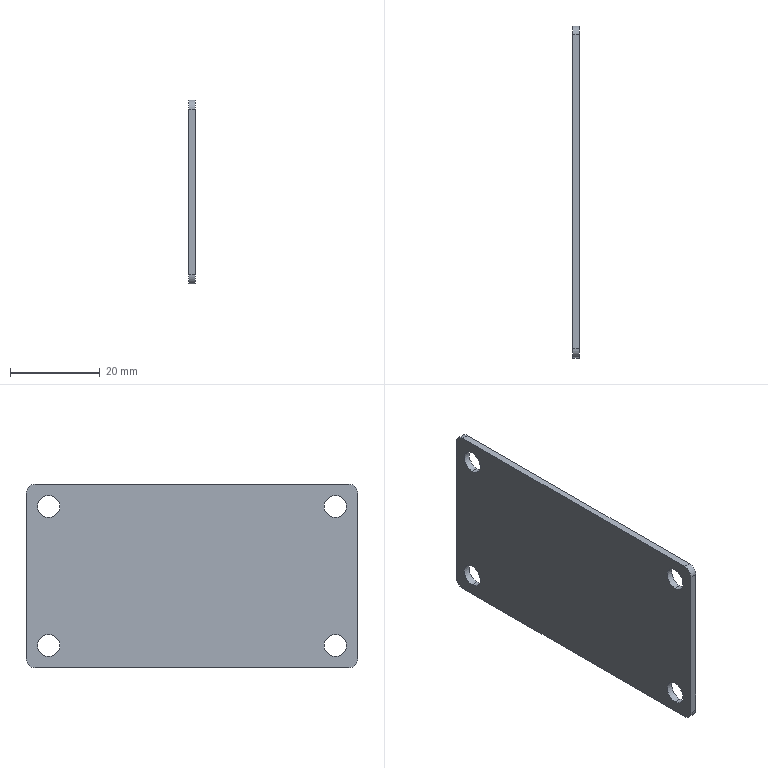Part | NX | features solid 2 | 1 solid | 18 faces | box 1.5 x 74 x 41 mm | volume 4428 mm3 | cylinder 12 | plane 6 | commonest cylinder face diameters 5 x8 4 x4
STEP:
#1=CARTESIAN_POINT('',(-328.,279.,-81.));
#2=VERTEX_POINT('',#1);
#3=CARTESIAN_POINT('',(-328.,277.,-83.));
#4=VERTEX_POINT('',#3);
#5=CARTESIAN_POINT('',(-328.,277.,-81.));
#6=DIRECTION('',(-1.,0.,0.));
#7=DIRECTION('',(0.,0.,-1.));
#8=AXIS2_PLACEMENT_3D('',#5,#6,#7);
#9=CIRCLE('',#8,2.);
#10=EDGE_CURVE('',#2,#4,#9,.T.);
#11=ORIENTED_EDGE('',*,*,#10,.F.);
#12=CARTESIAN_POINT('',(-326.5,279.,-81.));
#13=VERTEX_POINT('',#12);
#14=CARTESIAN_POINT('',(-328.,279.,-81.));
#15=DIRECTION('',(-1.,0.,0.));
#16=VECTOR('',#15,1000.);
#17=LINE('',#14,#16);
#18=EDGE_CURVE('',#13,#2,#17,.T.);
#19=ORIENTED_EDGE('',*,*,#18,.F.);
#20=CARTESIAN_POINT('',(-326.5,277.,-83.));
#21=VERTEX_POINT('',#20);
#22=CARTESIAN_POINT('',(-326.5,277.,-81.));
#23=DIRECTION('',(1.,0.,0.));
#24=DIRECTION('',(0.,0.,-1.));
#25=AXIS2_PLACEMENT_3D('',#22,#23,#24);
#26=CIRCLE('',#25,2.);
#27=EDGE_CURVE('',#21,#13,#26,.T.);
#28=ORIENTED_EDGE('',*,*,#27,.F.);
#29=CARTESIAN_POINT('',(-328.,277.,-83.));
#30=DIRECTION('',(1.,0.,0.));
#31=VECTOR('',#30,1000.);
#32=LINE('',#29,#31);
#33=EDGE_CURVE('',#4,#21,#32,.T.);
#34=ORIENTED_EDGE('',*,*,#33,.F.);
#35=EDGE_LOOP('',(#11,#19,#28,#34));
#36=FACE_BOUND('',#35,.T.);
#37=CARTESIAN_POINT('',(-328.,277.,-81.));
#38=DIRECTION('',(1.,0.,0.));
#39=DIRECTION('',(0.,0.,1.));
#40=AXIS2_PLACEMENT_3D('',#37,#38,#39);
#41=CYLINDRICAL_SURFACE('',#40,2.);
#42=ADVANCED_FACE('',(#36),#41,.T.);
#43=CARTESIAN_POINT('',(-328.,207.,-83.));
#44=VERTEX_POINT('',#43);
#45=CARTESIAN_POINT('',(-328.,205.,-81.));
#46=VERTEX_POINT('',#45);
#47=CARTESIAN_POINT('',(-328.,207.,-81.));
#48=DIRECTION('',(-1.,0.,0.));
#49=DIRECTION('',(0.,0.,-1.));
#50=AXIS2_PLACEMENT_3D('',#47,#48,#49);
#51=CIRCLE('',#50,2.);
#52=EDGE_CURVE('',#44,#46,#51,.T.);
#53=ORIENTED_EDGE('',*,*,#52,.F.);
#54=CARTESIAN_POINT('',(-326.5,207.,-83.));
#55=VERTEX_POINT('',#54);
#56=CARTESIAN_POINT('',(-328.,207.,-83.));
#57=DIRECTION('',(-1.,0.,0.));
#58=VECTOR('',#57,1000.);
#59=LINE('',#56,#58);
#60=EDGE_CURVE('',#55,#44,#59,.T.);
#61=ORIENTED_EDGE('',*,*,#60,.F.);
#62=CARTESIAN_POINT('',(-326.5,205.,-81.));
#63=VERTEX_POINT('',#62);
#64=CARTESIAN_POINT('',(-326.5,207.,-81.));
#65=DIRECTION('',(1.,0.,0.));
#66=DIRECTION('',(0.,0.,-1.));
#67=AXIS2_PLACEMENT_3D('',#64,#65,#66);
#68=CIRCLE('',#67,2.);
#69=EDGE_CURVE('',#63,#55,#68,.T.);
#70=ORIENTED_EDGE('',*,*,#69,.F.);
#71=CARTESIAN_POINT('',(-328.,205.,-81.));
#72=DIRECTION('',(1.,0.,0.));
#73=VECTOR('',#72,1000.);
#74=LINE('',#71,#73);
#75=EDGE_CURVE('',#46,#63,#74,.T.);
#76=ORIENTED_EDGE('',*,*,#75,.F.);
#77=EDGE_LOOP('',(#53,#61,#70,#76));
#78=FACE_BOUND('',#77,.T.);
#79=CARTESIAN_POINT('',(-328.,207.,-81.));
#80=DIRECTION('',(1.,0.,0.));
#81=DIRECTION('',(0.,0.,1.));
#82=AXIS2_PLACEMENT_3D('',#79,#80,#81);
#83=CYLINDRICAL_SURFACE('',#82,2.);
#84=ADVANCED_FACE('',(#78),#83,.T.);
#85=CARTESIAN_POINT('',(-328.,277.,-42.));
#86=VERTEX_POINT('',#85);
#87=CARTESIAN_POINT('',(-328.,279.,-44.));
#88=VERTEX_POINT('',#87);
#89=CARTESIAN_POINT('',(-328.,277.,-44.));
#90=DIRECTION('',(-1.,0.,0.));
#91=DIRECTION('',(0.,0.,-1.));
#92=AXIS2_PLACEMENT_3D('',#89,#90,#91);
#93=CIRCLE('',#92,2.);
#94=EDGE_CURVE('',#86,#88,#93,.T.);
#95=ORIENTED_EDGE('',*,*,#94,.F.);
#96=CARTESIAN_POINT('',(-326.5,277.,-42.));
#97=VERTEX_POINT('',#96);
#98=CARTESIAN_POINT('',(-328.,277.,-42.));
#99=DIRECTION('',(-1.,0.,0.));
#100=VECTOR('',#99,1000.);
#101=LINE('',#98,#100);
#102=EDGE_CURVE('',#97,#86,#101,.T.);
#103=ORIENTED_EDGE('',*,*,#102,.F.);
#104=CARTESIAN_POINT('',(-326.5,279.,-44.));
#105=VERTEX_POINT('',#104);
#106=CARTESIAN_POINT('',(-326.5,277.,-44.));
#107=DIRECTION('',(1.,0.,0.));
#108=DIRECTION('',(0.,0.,-1.));
#109=AXIS2_PLACEMENT_3D('',#106,#107,#108);
#110=CIRCLE('',#109,2.);
#111=EDGE_CURVE('',#105,#97,#110,.T.);
#112=ORIENTED_EDGE('',*,*,#111,.F.);
#113=CARTESIAN_POINT('',(-328.,279.,-44.));
#114=DIRECTION('',(1.,0.,0.));
#115=VECTOR('',#114,1000.);
#116=LINE('',#113,#115);
#117=EDGE_CURVE('',#88,#105,#116,.T.);
#118=ORIENTED_EDGE('',*,*,#117,.F.);
#119=EDGE_LOOP('',(#95,#103,#112,#118));
#120=FACE_BOUND('',#119,.T.);
#121=CARTESIAN_POINT('',(-328.,277.,-44.));
#122=DIRECTION('',(1.,0.,0.));
#123=DIRECTION('',(0.,0.,1.));
#124=AXIS2_PLACEMENT_3D('',#121,#122,#123);
#125=CYLINDRICAL_SURFACE('',#124,2.);
#126=ADVANCED_FACE('',(#120),#125,.T.);
#127=CARTESIAN_POINT('',(-328.,205.,-44.));
#128=VERTEX_POINT('',#127);
#129=CARTESIAN_POINT('',(-328.,207.,-42.));
#130=VERTEX_POINT('',#129);
#131=CARTESIAN_POINT('',(-328.,207.,-44.));
#132=DIRECTION('',(-1.,0.,0.));
#133=DIRECTION('',(0.,0.,-1.));
#134=AXIS2_PLACEMENT_3D('',#131,#132,#133);
#135=CIRCLE('',#134,2.);
#136=EDGE_CURVE('',#128,#130,#135,.T.);
#137=ORIENTED_EDGE('',*,*,#136,.F.);
#138=CARTESIAN_POINT('',(-326.5,205.,-44.));
#139=VERTEX_POINT('',#138);
#140=CARTESIAN_POINT('',(-328.,205.,-44.));
#141=DIRECTION('',(-1.,0.,0.));
#142=VECTOR('',#141,1000.);
#143=LINE('',#140,#142);
#144=EDGE_CURVE('',#139,#128,#143,.T.);
#145=ORIENTED_EDGE('',*,*,#144,.F.);
#146=CARTESIAN_POINT('',(-326.5,207.,-42.));
#147=VERTEX_POINT('',#146);
#148=CARTESIAN_POINT('',(-326.5,207.,-44.));
#149=DIRECTION('',(1.,0.,0.));
#150=DIRECTION('',(0.,0.,-1.));
#151=AXIS2_PLACEMENT_3D('',#148,#149,#150);
#152=CIRCLE('',#151,2.);
#153=EDGE_CURVE('',#147,#139,#152,.T.);
#154=ORIENTED_EDGE('',*,*,#153,.F.);
#155=CARTESIAN_POINT('',(-328.,207.,-42.));
#156=DIRECTION('',(1.,0.,0.));
#157=VECTOR('',#156,1000.);
#158=LINE('',#155,#157);
#159=EDGE_CURVE('',#130,#147,#158,.T.);
#160=ORIENTED_EDGE('',*,*,#159,.F.);
#161=EDGE_LOOP('',(#137,#145,#154,#160));
#162=FACE_BOUND('',#161,.T.);
#163=CARTESIAN_POINT('',(-328.,207.,-44.));
#164=DIRECTION('',(1.,0.,0.));
#165=DIRECTION('',(0.,0.,1.));
#166=AXIS2_PLACEMENT_3D('',#163,#164,#165);
#167=CYLINDRICAL_SURFACE('',#166,2.);
#168=ADVANCED_FACE('',(#162),#167,.T.);
#169=CARTESIAN_POINT('',(-326.5,274.,-49.5));
#170=VERTEX_POINT('',#169);
#171=CARTESIAN_POINT('',(-328.,274.,-49.5));
#172=VERTEX_POINT('',#171);
#173=CARTESIAN_POINT('',(-411.112,274.,-49.5));
#174=DIRECTION('',(1.,0.,0.));
#175=VECTOR('',#174,1000.);
#176=LINE('',#173,#175);
#177=EDGE_CURVE('',#170,#172,#176,.F.);
#178=ORIENTED_EDGE('',*,*,#177,.T.);
#179=CARTESIAN_POINT('',(-328.,274.,-44.5));
#180=VERTEX_POINT('',#179);
#181=CARTESIAN_POINT('',(-328.,274.,-47.));
#182=DIRECTION('',(-1.,0.,0.));
#183=DIRECTION('',(0.,0.,-1.));
#184=AXIS2_PLACEMENT_3D('',#181,#182,#183);
#185=CIRCLE('',#184,2.5);
#186=EDGE_CURVE('',#172,#180,#185,.T.);
#187=ORIENTED_EDGE('',*,*,#186,.T.);
#188=CARTESIAN_POINT('',(-326.5,274.,-44.5));
#189=VERTEX_POINT('',#188);
#190=CARTESIAN_POINT('',(-411.112,274.,-44.5));
#191=DIRECTION('',(1.,0.,0.));
#192=VECTOR('',#191,1000.);
#193=LINE('',#190,#192);
#194=EDGE_CURVE('',#180,#189,#193,.T.);
#195=ORIENTED_EDGE('',*,*,#194,.T.);
#196=CARTESIAN_POINT('',(-326.5,274.,-47.));
#197=DIRECTION('',(1.,0.,0.));
#198=DIRECTION('',(0.,-1.,0.));
#199=AXIS2_PLACEMENT_3D('',#196,#197,#198);
#200=CIRCLE('',#199,2.5);
#201=EDGE_CURVE('',#189,#170,#200,.T.);
#202=ORIENTED_EDGE('',*,*,#201,.T.);
#203=EDGE_LOOP('',(#178,#187,#195,#202));
#204=FACE_BOUND('',#203,.T.);
#205=CARTESIAN_POINT('',(-411.112,274.,-47.));
#206=DIRECTION('',(1.,0.,0.));
#207=DIRECTION('',(0.,0.,1.));
#208=AXIS2_PLACEMENT_3D('',#205,#206,#207);
#209=CYLINDRICAL_SURFACE('',#208,2.5);
#210=ADVANCED_FACE('',(#204),#209,.F.);
#211=CARTESIAN_POINT('',(-326.5,210.,-49.5));
#212=VERTEX_POINT('',#211);
#213=CARTESIAN_POINT('',(-328.,210.,-49.5));
#214=VERTEX_POINT('',#213);
#215=CARTESIAN_POINT('',(-411.112,210.,-49.5));
#216=DIRECTION('',(1.,0.,0.));
#217=VECTOR('',#216,1000.);
#218=LINE('',#215,#217);
#219=EDGE_CURVE('',#212,#214,#218,.F.);
#220=ORIENTED_EDGE('',*,*,#219,.T.);
#221=CARTESIAN_POINT('',(-328.,210.,-44.5));
#222=VERTEX_POINT('',#221);
#223=CARTESIAN_POINT('',(-328.,210.,-47.));
#224=DIRECTION('',(-1.,0.,0.));
#225=DIRECTION('',(0.,0.,-1.));
#226=AXIS2_PLACEMENT_3D('',#223,#224,#225);
#227=CIRCLE('',#226,2.5);
#228=EDGE_CURVE('',#214,#222,#227,.T.);
#229=ORIENTED_EDGE('',*,*,#228,.T.);
#230=CARTESIAN_POINT('',(-326.5,210.,-44.5));
#231=VERTEX_POINT('',#230);
#232=CARTESIAN_POINT('',(-411.112,210.,-44.5));
#233=DIRECTION('',(1.,0.,0.));
#234=VECTOR('',#233,1000.);
#235=LINE('',#232,#234);
#236=EDGE_CURVE('',#222,#231,#235,.T.);
#237=ORIENTED_EDGE('',*,*,#236,.T.);
#238=CARTESIAN_POINT('',(-326.5,210.,-47.));
#239=DIRECTION('',(1.,0.,0.));
#240=DIRECTION('',(0.,-1.,0.));
#241=AXIS2_PLACEMENT_3D('',#238,#239,#240);
#242=CIRCLE('',#241,2.5);
#243=EDGE_CURVE('',#231,#212,#242,.T.);
#244=ORIENTED_EDGE('',*,*,#243,.T.);
#245=EDGE_LOOP('',(#220,#229,#237,#244));
#246=FACE_BOUND('',#245,.T.);
#247=CARTESIAN_POINT('',(-411.112,210.,-47.));
#248=DIRECTION('',(1.,0.,0.));
#249=DIRECTION('',(0.,0.,1.));
#250=AXIS2_PLACEMENT_3D('',#247,#248,#249);
#251=CYLINDRICAL_SURFACE('',#250,2.5);
#252=ADVANCED_FACE('',(#246),#251,.F.);
#253=CARTESIAN_POINT('',(-328.,210.,-80.5));
#254=VERTEX_POINT('',#253);
#255=CARTESIAN_POINT('',(-326.5,210.,-80.5));
#256=VERTEX_POINT('',#255);
#257=CARTESIAN_POINT('',(-411.112,210.,-80.5));
#258=DIRECTION('',(1.,0.,0.));
#259=VECTOR('',#258,1000.);
#260=LINE('',#257,#259);
#261=EDGE_CURVE('',#254,#256,#260,.T.);
#262=ORIENTED_EDGE('',*,*,#261,.F.);
#263=CARTESIAN_POINT('',(-328.,210.,-75.5));
#264=VERTEX_POINT('',#263);
#265=CARTESIAN_POINT('',(-328.,210.,-78.));
#266=DIRECTION('',(-1.,0.,0.));
#267=DIRECTION('',(0.,0.,-1.));
#268=AXIS2_PLACEMENT_3D('',#265,#266,#267);
#269=CIRCLE('',#268,2.5);
#270=EDGE_CURVE('',#254,#264,#269,.T.);
#271=ORIENTED_EDGE('',*,*,#270,.T.);
#272=CARTESIAN_POINT('',(-326.5,210.,-75.5));
#273=VERTEX_POINT('',#272);
#274=CARTESIAN_POINT('',(-411.112,210.,-75.5));
#275=DIRECTION('',(1.,0.,0.));
#276=VECTOR('',#275,1000.);
#277=LINE('',#274,#276);
#278=EDGE_CURVE('',#273,#264,#277,.F.);
#279=ORIENTED_EDGE('',*,*,#278,.F.);
#280=CARTESIAN_POINT('',(-326.5,210.,-78.));
#281=DIRECTION('',(1.,0.,0.));
#282=DIRECTION('',(0.,-1.,0.));
#283=AXIS2_PLACEMENT_3D('',#280,#281,#282);
#284=CIRCLE('',#283,2.5);
#285=EDGE_CURVE('',#273,#256,#284,.T.);
#286=ORIENTED_EDGE('',*,*,#285,.T.);
#287=EDGE_LOOP('',(#262,#271,#279,#286));
#288=FACE_BOUND('',#287,.T.);
#289=CARTESIAN_POINT('',(-411.112,210.,-78.));
#290=DIRECTION('',(1.,0.,0.));
#291=DIRECTION('',(0.,0.,1.));
#292=AXIS2_PLACEMENT_3D('',#289,#290,#291);
#293=CYLINDRICAL_SURFACE('',#292,2.5);
#294=ADVANCED_FACE('',(#288),#293,.F.);
#295=CARTESIAN_POINT('',(-326.5,274.,-80.5));
#296=VERTEX_POINT('',#295);
#297=CARTESIAN_POINT('',(-328.,274.,-80.5));
#298=VERTEX_POINT('',#297);
#299=CARTESIAN_POINT('',(-411.112,274.,-80.5));
#300=DIRECTION('',(1.,0.,0.));
#301=VECTOR('',#300,1000.);
#302=LINE('',#299,#301);
#303=EDGE_CURVE('',#296,#298,#302,.F.);
#304=ORIENTED_EDGE('',*,*,#303,.T.);
#305=CARTESIAN_POINT('',(-328.,274.,-75.5));
#306=VERTEX_POINT('',#305);
#307=CARTESIAN_POINT('',(-328.,274.,-78.));
#308=DIRECTION('',(-1.,0.,0.));
#309=DIRECTION('',(0.,0.,-1.));
#310=AXIS2_PLACEMENT_3D('',#307,#308,#309);
#311=CIRCLE('',#310,2.5);
#312=EDGE_CURVE('',#298,#306,#311,.T.);
#313=ORIENTED_EDGE('',*,*,#312,.T.);
#314=CARTESIAN_POINT('',(-326.5,274.,-75.5));
#315=VERTEX_POINT('',#314);
#316=CARTESIAN_POINT('',(-411.112,274.,-75.5));
#317=DIRECTION('',(1.,0.,0.));
#318=VECTOR('',#317,1000.);
#319=LINE('',#316,#318);
#320=EDGE_CURVE('',#306,#315,#319,.T.);
#321=ORIENTED_EDGE('',*,*,#320,.T.);
#322=CARTESIAN_POINT('',(-326.5,274.,-78.));
#323=DIRECTION('',(1.,0.,0.));
#324=DIRECTION('',(0.,-1.,0.));
#325=AXIS2_PLACEMENT_3D('',#322,#323,#324);
#326=CIRCLE('',#325,2.5);
#327=EDGE_CURVE('',#315,#296,#326,.T.);
#328=ORIENTED_EDGE('',*,*,#327,.T.);
#329=EDGE_LOOP('',(#304,#313,#321,#328));
#330=FACE_BOUND('',#329,.T.);
#331=CARTESIAN_POINT('',(-411.112,274.,-78.));
#332=DIRECTION('',(1.,0.,0.));
#333=DIRECTION('',(0.,0.,1.));
#334=AXIS2_PLACEMENT_3D('',#331,#332,#333);
#335=CYLINDRICAL_SURFACE('',#334,2.5);
#336=ADVANCED_FACE('',(#330),#335,.F.);
#337=ORIENTED_EDGE('',*,*,#327,.F.);
#338=CARTESIAN_POINT('',(-326.5,274.,-78.));
#339=DIRECTION('',(1.,0.,0.));
#340=DIRECTION('',(0.,-1.,0.));
#341=AXIS2_PLACEMENT_3D('',#338,#339,#340);
#342=CIRCLE('',#341,2.5);
#343=EDGE_CURVE('',#296,#315,#342,.T.);
#344=ORIENTED_EDGE('',*,*,#343,.F.);
#345=EDGE_LOOP('',(#337,#344));
#346=FACE_BOUND('',#345,.T.);
#347=ORIENTED_EDGE('',*,*,#285,.F.);
#348=CARTESIAN_POINT('',(-326.5,210.,-78.));
#349=DIRECTION('',(1.,0.,0.));
#350=DIRECTION('',(0.,-1.,0.));
#351=AXIS2_PLACEMENT_3D('',#348,#349,#350);
#352=CIRCLE('',#351,2.5);
#353=EDGE_CURVE('',#256,#273,#352,.T.);
#354=ORIENTED_EDGE('',*,*,#353,.F.);
#355=EDGE_LOOP('',(#347,#354));
#356=FACE_BOUND('',#355,.T.);
#357=ORIENTED_EDGE('',*,*,#243,.F.);
#358=CARTESIAN_POINT('',(-326.5,210.,-47.));
#359=DIRECTION('',(1.,0.,0.));
#360=DIRECTION('',(0.,-1.,0.));
#361=AXIS2_PLACEMENT_3D('',#358,#359,#360);
#362=CIRCLE('',#361,2.5);
#363=EDGE_CURVE('',#212,#231,#362,.T.);
#364=ORIENTED_EDGE('',*,*,#363,.F.);
#365=EDGE_LOOP('',(#357,#364));
#366=FACE_BOUND('',#365,.T.);
#367=ORIENTED_EDGE('',*,*,#201,.F.);
#368=CARTESIAN_POINT('',(-326.5,274.,-47.));
#369=DIRECTION('',(1.,0.,0.));
#370=DIRECTION('',(0.,-1.,0.));
#371=AXIS2_PLACEMENT_3D('',#368,#369,#370);
#372=CIRCLE('',#371,2.5);
#373=EDGE_CURVE('',#170,#189,#372,.T.);
#374=ORIENTED_EDGE('',*,*,#373,.F.);
#375=EDGE_LOOP('',(#367,#374));
#376=FACE_BOUND('',#375,.T.);
#377=CARTESIAN_POINT('',(-326.5,205.,-42.));
#378=DIRECTION('',(0.,1.,0.));
#379=VECTOR('',#378,1000.);
#380=LINE('',#377,#379);
#381=EDGE_CURVE('',#147,#97,#380,.T.);
#382=ORIENTED_EDGE('',*,*,#381,.F.);
#383=ORIENTED_EDGE('',*,*,#153,.T.);
#384=CARTESIAN_POINT('',(-326.5,205.,-83.));
#385=DIRECTION('',(0.,0.,1.));
#386=VECTOR('',#385,1000.);
#387=LINE('',#384,#386);
#388=EDGE_CURVE('',#63,#139,#387,.T.);
#389=ORIENTED_EDGE('',*,*,#388,.F.);
#390=ORIENTED_EDGE('',*,*,#69,.T.);
#391=CARTESIAN_POINT('',(-326.5,279.,-83.));
#392=DIRECTION('',(0.,-1.,0.));
#393=VECTOR('',#392,1000.);
#394=LINE('',#391,#393);
#395=EDGE_CURVE('',#21,#55,#394,.T.);
#396=ORIENTED_EDGE('',*,*,#395,.F.);
#397=ORIENTED_EDGE('',*,*,#27,.T.);
#398=CARTESIAN_POINT('',(-326.5,279.,-42.));
#399=DIRECTION('',(0.,0.,-1.));
#400=VECTOR('',#399,1000.);
#401=LINE('',#398,#400);
#402=EDGE_CURVE('',#105,#13,#401,.T.);
#403=ORIENTED_EDGE('',*,*,#402,.F.);
#404=ORIENTED_EDGE('',*,*,#111,.T.);
#405=EDGE_LOOP('',(#382,#383,#389,#390,#396,#397,#403,#404));
#406=FACE_BOUND('',#405,.T.);
#407=CARTESIAN_POINT('',(-326.5,242.,-62.5));
#408=DIRECTION('',(-1.,0.,0.));
#409=DIRECTION('',(0.,0.,1.));
#410=AXIS2_PLACEMENT_3D('',#407,#408,#409);
#411=PLANE('',#410);
#412=ADVANCED_FACE('',(#346,#356,#366,#376,#406),#411,.F.);
#413=CARTESIAN_POINT('',(-328.,274.,-78.));
#414=DIRECTION('',(-1.,0.,0.));
#415=DIRECTION('',(0.,0.,-1.));
#416=AXIS2_PLACEMENT_3D('',#413,#414,#415);
#417=CIRCLE('',#416,2.5);
#418=EDGE_CURVE('',#306,#298,#417,.T.);
#419=ORIENTED_EDGE('',*,*,#418,.F.);
#420=ORIENTED_EDGE('',*,*,#312,.F.);
#421=EDGE_LOOP('',(#419,#420));
#422=FACE_BOUND('',#421,.T.);
#423=CARTESIAN_POINT('',(-328.,210.,-78.));
#424=DIRECTION('',(-1.,0.,0.));
#425=DIRECTION('',(0.,0.,-1.));
#426=AXIS2_PLACEMENT_3D('',#423,#424,#425);
#427=CIRCLE('',#426,2.5);
#428=EDGE_CURVE('',#264,#254,#427,.T.);
#429=ORIENTED_EDGE('',*,*,#428,.F.);
#430=ORIENTED_EDGE('',*,*,#270,.F.);
#431=EDGE_LOOP('',(#429,#430));
#432=FACE_BOUND('',#431,.T.);
#433=CARTESIAN_POINT('',(-328.,210.,-47.));
#434=DIRECTION('',(-1.,0.,0.));
#435=DIRECTION('',(0.,0.,-1.));
#436=AXIS2_PLACEMENT_3D('',#433,#434,#435);
#437=CIRCLE('',#436,2.5);
#438=EDGE_CURVE('',#222,#214,#437,.T.);
#439=ORIENTED_EDGE('',*,*,#438,.F.);
#440=ORIENTED_EDGE('',*,*,#228,.F.);
#441=EDGE_LOOP('',(#439,#440));
#442=FACE_BOUND('',#441,.T.);
#443=CARTESIAN_POINT('',(-328.,274.,-47.));
#444=DIRECTION('',(-1.,0.,0.));
#445=DIRECTION('',(0.,0.,-1.));
#446=AXIS2_PLACEMENT_3D('',#443,#444,#445);
#447=CIRCLE('',#446,2.5);
#448=EDGE_CURVE('',#180,#172,#447,.T.);
#449=ORIENTED_EDGE('',*,*,#448,.F.);
#450=ORIENTED_EDGE('',*,*,#186,.F.);
#451=EDGE_LOOP('',(#449,#450));
#452=FACE_BOUND('',#451,.T.);
#453=CARTESIAN_POINT('',(-328.,205.,-83.));
#454=DIRECTION('',(0.,0.,1.));
#455=VECTOR('',#454,1000.);
#456=LINE('',#453,#455);
#457=EDGE_CURVE('',#46,#128,#456,.T.);
#458=ORIENTED_EDGE('',*,*,#457,.T.);
#459=ORIENTED_EDGE('',*,*,#136,.T.);
#460=CARTESIAN_POINT('',(-328.,205.,-42.));
#461=DIRECTION('',(0.,1.,0.));
#462=VECTOR('',#461,1000.);
#463=LINE('',#460,#462);
#464=EDGE_CURVE('',#130,#86,#463,.T.);
#465=ORIENTED_EDGE('',*,*,#464,.T.);
#466=ORIENTED_EDGE('',*,*,#94,.T.);
#467=CARTESIAN_POINT('',(-328.,279.,-42.));
#468=DIRECTION('',(0.,0.,-1.));
#469=VECTOR('',#468,1000.);
#470=LINE('',#467,#469);
#471=EDGE_CURVE('',#88,#2,#470,.T.);
#472=ORIENTED_EDGE('',*,*,#471,.T.);
#473=ORIENTED_EDGE('',*,*,#10,.T.);
#474=CARTESIAN_POINT('',(-328.,279.,-83.));
#475=DIRECTION('',(0.,-1.,0.));
#476=VECTOR('',#475,1000.);
#477=LINE('',#474,#476);
#478=EDGE_CURVE('',#4,#44,#477,.T.);
#479=ORIENTED_EDGE('',*,*,#478,.T.);
#480=ORIENTED_EDGE('',*,*,#52,.T.);
#481=EDGE_LOOP('',(#458,#459,#465,#466,#472,#473,#479,#480));
#482=FACE_BOUND('',#481,.T.);
#483=CARTESIAN_POINT('',(-328.,242.,-62.5));
#484=DIRECTION('',(-1.,0.,0.));
#485=DIRECTION('',(0.,0.,1.));
#486=AXIS2_PLACEMENT_3D('',#483,#484,#485);
#487=PLANE('',#486);
#488=ADVANCED_FACE('',(#422,#432,#442,#452,#482),#487,.T.);
#489=ORIENTED_EDGE('',*,*,#395,.T.);
#490=ORIENTED_EDGE('',*,*,#60,.T.);
#491=ORIENTED_EDGE('',*,*,#478,.F.);
#492=ORIENTED_EDGE('',*,*,#33,.T.);
#493=EDGE_LOOP('',(#489,#490,#491,#492));
#494=FACE_BOUND('',#493,.T.);
#495=CARTESIAN_POINT('',(-328.,279.,-83.));
#496=DIRECTION('',(0.,0.,1.));
#497=DIRECTION('',(0.,-1.,0.));
#498=AXIS2_PLACEMENT_3D('',#495,#496,#497);
#499=PLANE('',#498);
#500=ADVANCED_FACE('',(#494),#499,.F.);
#501=ORIENTED_EDGE('',*,*,#471,.F.);
#502=ORIENTED_EDGE('',*,*,#117,.T.);
#503=ORIENTED_EDGE('',*,*,#402,.T.);
#504=ORIENTED_EDGE('',*,*,#18,.T.);
#505=EDGE_LOOP('',(#501,#502,#503,#504));
#506=FACE_BOUND('',#505,.T.);
#507=CARTESIAN_POINT('',(-328.,279.,-42.));
#508=DIRECTION('',(0.,-1.,0.));
#509=DIRECTION('',(-1.,0.,0.));
#510=AXIS2_PLACEMENT_3D('',#507,#508,#509);
#511=PLANE('',#510);
#512=ADVANCED_FACE('',(#506),#511,.F.);
#513=ORIENTED_EDGE('',*,*,#464,.F.);
#514=ORIENTED_EDGE('',*,*,#159,.T.);
#515=ORIENTED_EDGE('',*,*,#381,.T.);
#516=ORIENTED_EDGE('',*,*,#102,.T.);
#517=EDGE_LOOP('',(#513,#514,#515,#516));
#518=FACE_BOUND('',#517,.T.);
#519=CARTESIAN_POINT('',(-328.,205.,-42.));
#520=DIRECTION('',(0.,0.,-1.));
#521=DIRECTION('',(0.,-1.,0.));
#522=AXIS2_PLACEMENT_3D('',#519,#520,#521);
#523=PLANE('',#522);
#524=ADVANCED_FACE('',(#518),#523,.F.);
#525=ORIENTED_EDGE('',*,*,#388,.T.);
#526=ORIENTED_EDGE('',*,*,#144,.T.);
#527=ORIENTED_EDGE('',*,*,#457,.F.);
#528=ORIENTED_EDGE('',*,*,#75,.T.);
#529=EDGE_LOOP('',(#525,#526,#527,#528));
#530=FACE_BOUND('',#529,.T.);
#531=CARTESIAN_POINT('',(-328.,205.,-83.));
#532=DIRECTION('',(0.,1.,0.));
#533=DIRECTION('',(0.,0.,-1.));
#534=AXIS2_PLACEMENT_3D('',#531,#532,#533);
#535=PLANE('',#534);
#536=ADVANCED_FACE('',(#530),#535,.F.);
#537=ORIENTED_EDGE('',*,*,#418,.T.);
#538=ORIENTED_EDGE('',*,*,#303,.F.);
#539=ORIENTED_EDGE('',*,*,#343,.T.);
#540=ORIENTED_EDGE('',*,*,#320,.F.);
#541=EDGE_LOOP('',(#537,#538,#539,#540));
#542=FACE_BOUND('',#541,.T.);
#543=CARTESIAN_POINT('',(-411.112,274.,-78.));
#544=DIRECTION('',(1.,0.,0.));
#545=DIRECTION('',(0.,0.,1.));
#546=AXIS2_PLACEMENT_3D('',#543,#544,#545);
#547=CYLINDRICAL_SURFACE('',#546,2.5);
#548=ADVANCED_FACE('',(#542),#547,.F.);
#549=ORIENTED_EDGE('',*,*,#428,.T.);
#550=ORIENTED_EDGE('',*,*,#261,.T.);
#551=ORIENTED_EDGE('',*,*,#353,.T.);
#552=ORIENTED_EDGE('',*,*,#278,.T.);
#553=EDGE_LOOP('',(#549,#550,#551,#552));
#554=FACE_BOUND('',#553,.T.);
#555=CARTESIAN_POINT('',(-411.112,210.,-78.));
#556=DIRECTION('',(1.,0.,0.));
#557=DIRECTION('',(0.,0.,1.));
#558=AXIS2_PLACEMENT_3D('',#555,#556,#557);
#559=CYLINDRICAL_SURFACE('',#558,2.5);
#560=ADVANCED_FACE('',(#554),#559,.F.);
#561=ORIENTED_EDGE('',*,*,#438,.T.);
#562=ORIENTED_EDGE('',*,*,#219,.F.);
#563=ORIENTED_EDGE('',*,*,#363,.T.);
#564=ORIENTED_EDGE('',*,*,#236,.F.);
#565=EDGE_LOOP('',(#561,#562,#563,#564));
#566=FACE_BOUND('',#565,.T.);
#567=CARTESIAN_POINT('',(-411.112,210.,-47.));
#568=DIRECTION('',(1.,0.,0.));
#569=DIRECTION('',(0.,0.,1.));
#570=AXIS2_PLACEMENT_3D('',#567,#568,#569);
#571=CYLINDRICAL_SURFACE('',#570,2.5);
#572=ADVANCED_FACE('',(#566),#571,.F.);
#573=ORIENTED_EDGE('',*,*,#448,.T.);
#574=ORIENTED_EDGE('',*,*,#177,.F.);
#575=ORIENTED_EDGE('',*,*,#373,.T.);
#576=ORIENTED_EDGE('',*,*,#194,.F.);
#577=EDGE_LOOP('',(#573,#574,#575,#576));
#578=FACE_BOUND('',#577,.T.);
#579=CARTESIAN_POINT('',(-411.112,274.,-47.));
#580=DIRECTION('',(1.,0.,0.));
#581=DIRECTION('',(0.,0.,1.));
#582=AXIS2_PLACEMENT_3D('',#579,#580,#581);
#583=CYLINDRICAL_SURFACE('',#582,2.5);
#584=ADVANCED_FACE('',(#578),#583,.F.);
#585=CLOSED_SHELL('',(#42,#84,#126,#168,#210,#252,#294,#336,#412,#488,#500,#512,#524,#536,#548,#560,#572,#584));
#586=MANIFOLD_SOLID_BREP('',#585);
#587=(LENGTH_UNIT()NAMED_UNIT(*)SI_UNIT(.MILLI.,.METRE.));
#588=UNCERTAINTY_MEASURE_WITH_UNIT(LENGTH_MEASURE(0.00001),#587,'','');
#589=(NAMED_UNIT(*)PLANE_ANGLE_UNIT()SI_UNIT($,.RADIAN.));
#590=(NAMED_UNIT(*)SI_UNIT($,.STERADIAN.)SOLID_ANGLE_UNIT());
#591=(GEOMETRIC_REPRESENTATION_CONTEXT(3)GLOBAL_UNCERTAINTY_ASSIGNED_CONTEXT((#588))GLOBAL_UNIT_ASSIGNED_CONTEXT((#587,#589,#590))REPRESENTATION_CONTEXT('',''));
#592=ADVANCED_BREP_SHAPE_REPRESENTATION('',(#586),#591);